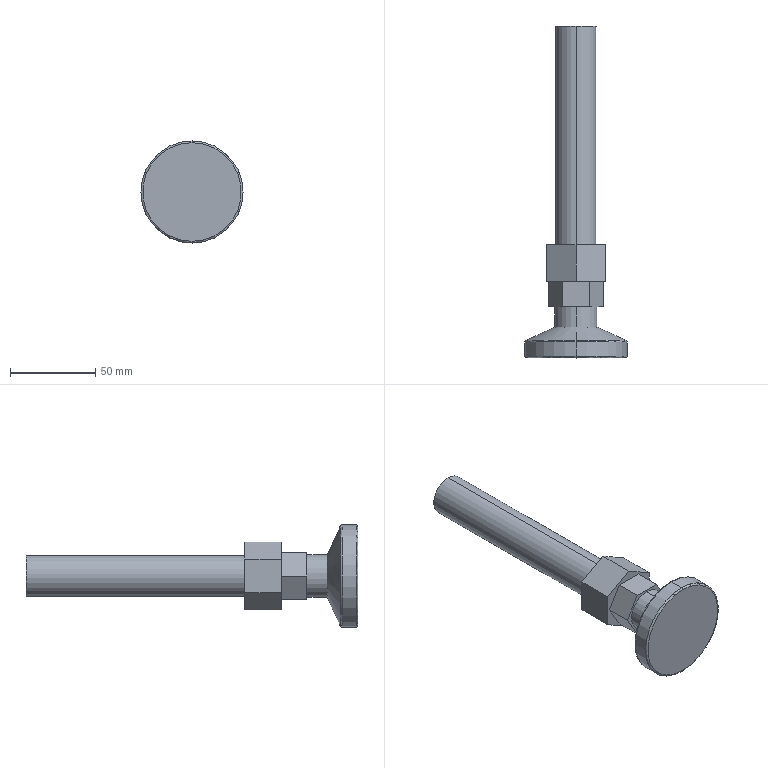Part | STEP file | All-carbon-steel swivel foot KCUF M24-150-60 | 1 solid | 29 faces | box 60 x 195 x 60 mm | volume 136685 mm3 | plane 17 | cylinder 6 | torus 4 | cone 2 | commonest cylinder face diameters 24 x2 25.261 x2 60 x2